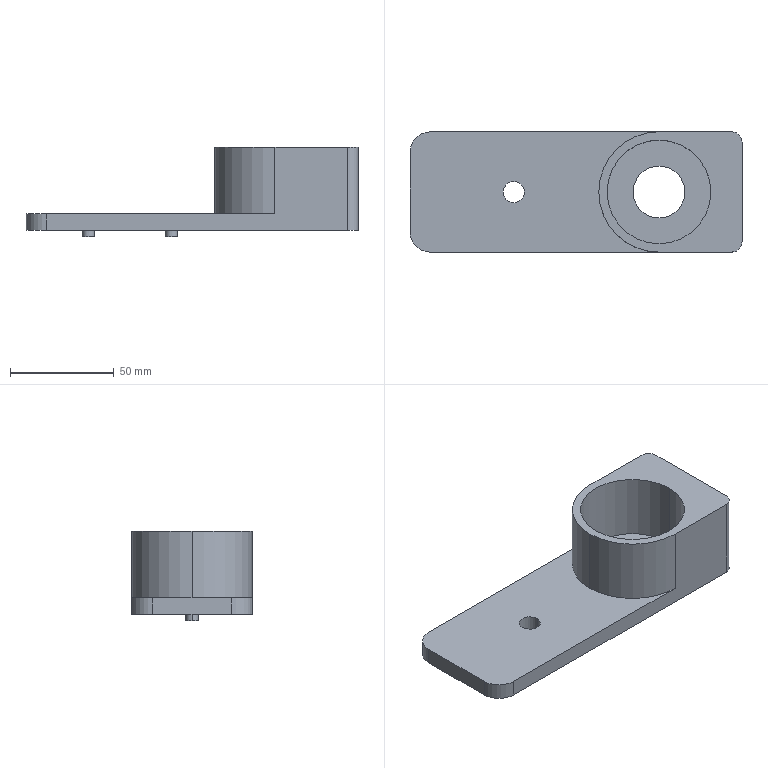Part | STEP file | Stop sleeve QY-1-25 | 1 solid | 42 faces | box 160 x 58 x 43 mm | volume 121520 mm3 | cylinder 24 | plane 10 | cone 8 | commonest cylinder face diameters 5 x8 6 x4 10 x2 10.2 x2 20 x2 25 x2